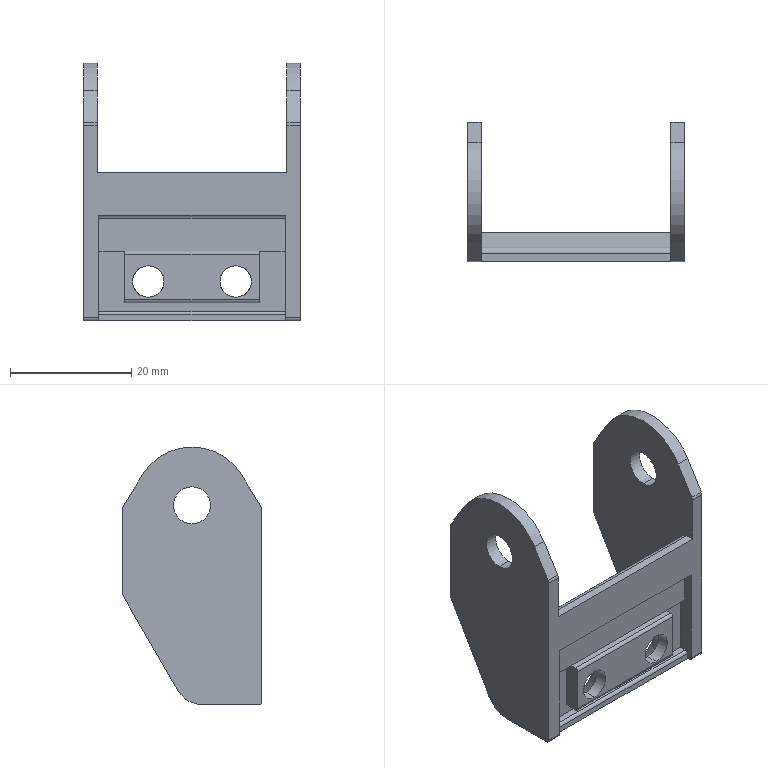Part | SolidWorks | features BaseBody 1 | 1 solid | 61 faces | box 35.7 x 23 x 42.499 mm | volume 5565 mm3 | plane 32 | cylinder 25 | cone 4 | commonest cylinder face diameters 2 x7 1 x6 5.2 x4 6.1 x4 10 x2 19.2 x2